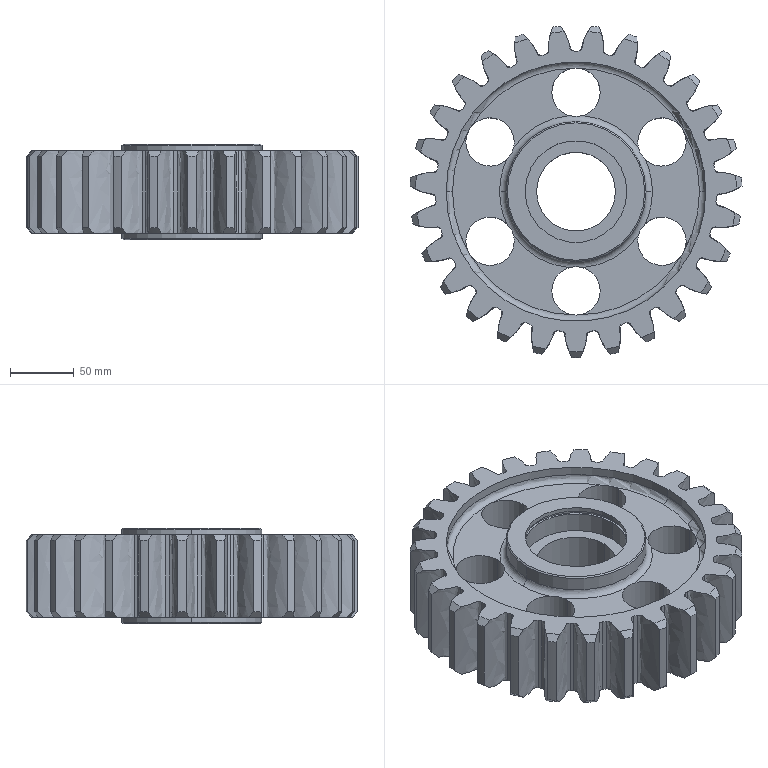Part | SolidWorks | features ICE 6, Chamfer 5, CirPattern 2, MirrorPattern 2, Extrusion 1, RefAxis 1, RevCut 1 | 1 solid | 230 faces | box 260.857 x 260.456 x 75 mm | volume 1917959 mm3 | cylinder 88 | cone 58 | spline 54 | plane 22 | torus 8 | commonest cylinder face diameters 220.5 x27 261 x27 38 x12 80 x8 83.5 x4 110 x4